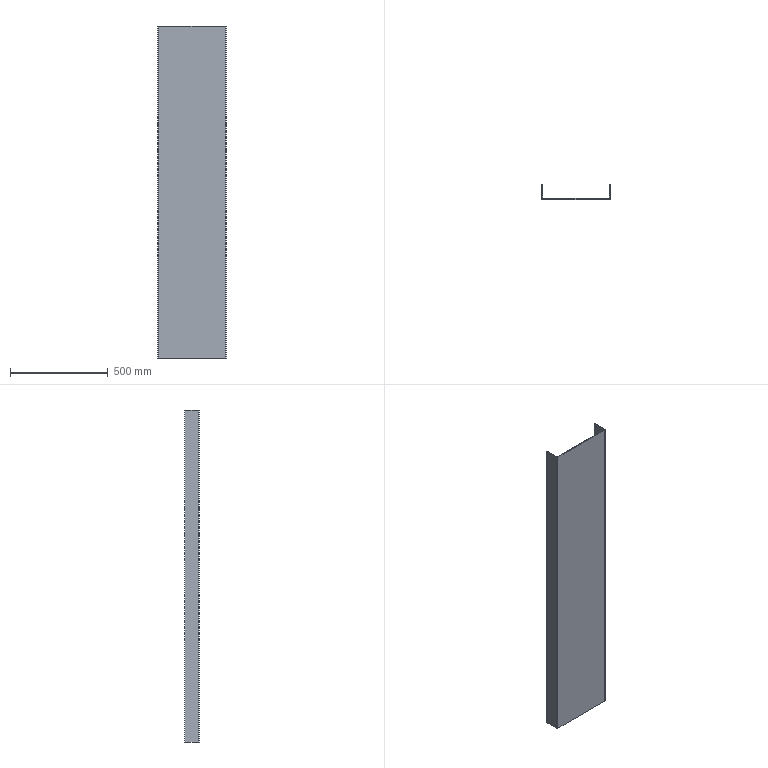Part | STEP file | Sheet metal 11 | 1 solid | 22 faces | box 350 x 75 x 1700 mm | volume 3328088 mm3 | plane 18 | cylinder 4 | commonest cylinder face diameters 2 x2 10 x2
STEP:
#1=CARTESIAN_POINT('',(-170.,-4.,850.));
#2=VERTEX_POINT('',#1);
#3=CARTESIAN_POINT('',(-170.,-4.,-850.));
#4=VERTEX_POINT('',#3);
#5=CARTESIAN_POINT('',(-170.,-4.,850.));
#6=DIRECTION('',(0.,0.,-1.));
#7=VECTOR('',#6,1000.);
#8=LINE('',#5,#7);
#9=EDGE_CURVE('',#2,#4,#8,.T.);
#10=ORIENTED_EDGE('',*,*,#9,.T.);
#11=CARTESIAN_POINT('',(170.,-4.,-850.));
#12=VERTEX_POINT('',#11);
#13=CARTESIAN_POINT('',(-175.,-4.,-850.));
#14=DIRECTION('',(-1.,0.,0.));
#15=VECTOR('',#14,1000.);
#16=LINE('',#13,#15);
#17=EDGE_CURVE('',#12,#4,#16,.T.);
#18=ORIENTED_EDGE('',*,*,#17,.F.);
#19=CARTESIAN_POINT('',(170.,-4.,850.));
#20=VERTEX_POINT('',#19);
#21=CARTESIAN_POINT('',(170.,-4.,-850.));
#22=DIRECTION('',(0.,0.,1.));
#23=VECTOR('',#22,1000.);
#24=LINE('',#21,#23);
#25=EDGE_CURVE('',#12,#20,#24,.T.);
#26=ORIENTED_EDGE('',*,*,#25,.T.);
#27=CARTESIAN_POINT('',(-175.,-4.,850.));
#28=DIRECTION('',(1.,0.,0.));
#29=VECTOR('',#28,1000.);
#30=LINE('',#27,#29);
#31=EDGE_CURVE('',#2,#20,#30,.T.);
#32=ORIENTED_EDGE('',*,*,#31,.F.);
#33=EDGE_LOOP('',(#10,#18,#26,#32));
#34=FACE_OUTER_BOUND('',#33,.T.);
#35=CARTESIAN_POINT('',(0.,-4.,0.));
#36=DIRECTION('',(0.,1.,0.));
#37=DIRECTION('',(0.,0.,1.));
#38=AXIS2_PLACEMENT_3D('',#35,#36,#37);
#39=PLANE('',#38);
#40=ADVANCED_FACE('',(#34),#39,.F.);
#41=CARTESIAN_POINT('',(170.,0.,-850.));
#42=VERTEX_POINT('',#41);
#43=CARTESIAN_POINT('',(-170.,0.,-850.));
#44=VERTEX_POINT('',#43);
#45=CARTESIAN_POINT('',(-175.,0.,-850.));
#46=DIRECTION('',(-1.,0.,0.));
#47=VECTOR('',#46,1000.);
#48=LINE('',#45,#47);
#49=EDGE_CURVE('',#42,#44,#48,.T.);
#50=ORIENTED_EDGE('',*,*,#49,.T.);
#51=CARTESIAN_POINT('',(-170.,0.,850.));
#52=VERTEX_POINT('',#51);
#53=CARTESIAN_POINT('',(-170.,0.,850.));
#54=DIRECTION('',(0.,0.,-1.));
#55=VECTOR('',#54,1000.);
#56=LINE('',#53,#55);
#57=EDGE_CURVE('',#52,#44,#56,.T.);
#58=ORIENTED_EDGE('',*,*,#57,.F.);
#59=CARTESIAN_POINT('',(170.,0.,850.));
#60=VERTEX_POINT('',#59);
#61=CARTESIAN_POINT('',(-175.,0.,850.));
#62=DIRECTION('',(1.,0.,0.));
#63=VECTOR('',#62,1000.);
#64=LINE('',#61,#63);
#65=EDGE_CURVE('',#52,#60,#64,.T.);
#66=ORIENTED_EDGE('',*,*,#65,.T.);
#67=CARTESIAN_POINT('',(170.,0.,-850.));
#68=DIRECTION('',(0.,0.,1.));
#69=VECTOR('',#68,1000.);
#70=LINE('',#67,#69);
#71=EDGE_CURVE('',#42,#60,#70,.T.);
#72=ORIENTED_EDGE('',*,*,#71,.F.);
#73=EDGE_LOOP('',(#50,#58,#66,#72));
#74=FACE_OUTER_BOUND('',#73,.T.);
#75=CARTESIAN_POINT('',(0.,0.,0.));
#76=DIRECTION('',(0.,1.,0.));
#77=DIRECTION('',(0.,0.,1.));
#78=AXIS2_PLACEMENT_3D('',#75,#76,#77);
#79=PLANE('',#78);
#80=ADVANCED_FACE('',(#74),#79,.T.);
#81=ORIENTED_EDGE('',*,*,#65,.F.);
#82=CARTESIAN_POINT('',(-170.,0.,850.));
#83=DIRECTION('',(0.,-1.,0.));
#84=VECTOR('',#83,1000.);
#85=LINE('',#82,#84);
#86=EDGE_CURVE('',#52,#2,#85,.T.);
#87=ORIENTED_EDGE('',*,*,#86,.T.);
#88=ORIENTED_EDGE('',*,*,#31,.T.);
#89=CARTESIAN_POINT('',(170.,0.,850.));
#90=DIRECTION('',(0.,-1.,0.));
#91=VECTOR('',#90,1000.);
#92=LINE('',#89,#91);
#93=EDGE_CURVE('',#60,#20,#92,.T.);
#94=ORIENTED_EDGE('',*,*,#93,.F.);
#95=EDGE_LOOP('',(#81,#87,#88,#94));
#96=FACE_OUTER_BOUND('',#95,.T.);
#97=CARTESIAN_POINT('',(-175.,-4.,850.));
#98=DIRECTION('',(0.,0.,1.));
#99=DIRECTION('',(1.,0.,0.));
#100=AXIS2_PLACEMENT_3D('',#97,#98,#99);
#101=PLANE('',#100);
#102=ADVANCED_FACE('',(#96),#101,.T.);
#103=CARTESIAN_POINT('',(-170.,0.,-850.));
#104=DIRECTION('',(0.,-1.,0.));
#105=VECTOR('',#104,1000.);
#106=LINE('',#103,#105);
#107=EDGE_CURVE('',#44,#4,#106,.T.);
#108=ORIENTED_EDGE('',*,*,#107,.F.);
#109=ORIENTED_EDGE('',*,*,#49,.F.);
#110=CARTESIAN_POINT('',(170.,0.,-850.));
#111=DIRECTION('',(0.,-1.,0.));
#112=VECTOR('',#111,1000.);
#113=LINE('',#110,#112);
#114=EDGE_CURVE('',#42,#12,#113,.T.);
#115=ORIENTED_EDGE('',*,*,#114,.T.);
#116=ORIENTED_EDGE('',*,*,#17,.T.);
#117=EDGE_LOOP('',(#108,#109,#115,#116));
#118=FACE_OUTER_BOUND('',#117,.T.);
#119=CARTESIAN_POINT('',(-175.,-4.,-850.));
#120=DIRECTION('',(0.,0.,-1.));
#121=DIRECTION('',(-1.,0.,0.));
#122=AXIS2_PLACEMENT_3D('',#119,#120,#121);
#123=PLANE('',#122);
#124=ADVANCED_FACE('',(#118),#123,.T.);
#125=CARTESIAN_POINT('',(171.,1.,850.));
#126=VERTEX_POINT('',#125);
#127=CARTESIAN_POINT('',(175.,1.,850.));
#128=VERTEX_POINT('',#127);
#129=CARTESIAN_POINT('',(175.,1.,850.));
#130=DIRECTION('',(1.,0.,0.));
#131=VECTOR('',#130,1000.);
#132=LINE('',#129,#131);
#133=EDGE_CURVE('',#126,#128,#132,.T.);
#134=ORIENTED_EDGE('',*,*,#133,.F.);
#135=CARTESIAN_POINT('',(170.,1.,850.));
#136=DIRECTION('',(0.,0.,1.));
#137=DIRECTION('',(-1.,0.,0.));
#138=AXIS2_PLACEMENT_3D('',#135,#136,#137);
#139=CIRCLE('',#138,1.);
#140=EDGE_CURVE('',#60,#126,#139,.T.);
#141=ORIENTED_EDGE('',*,*,#140,.F.);
#142=ORIENTED_EDGE('',*,*,#93,.T.);
#143=CARTESIAN_POINT('',(170.,1.,850.));
#144=DIRECTION('',(0.,0.,1.));
#145=DIRECTION('',(-1.,0.,0.));
#146=AXIS2_PLACEMENT_3D('',#143,#144,#145);
#147=CIRCLE('',#146,5.);
#148=EDGE_CURVE('',#20,#128,#147,.T.);
#149=ORIENTED_EDGE('',*,*,#148,.T.);
#150=EDGE_LOOP('',(#134,#141,#142,#149));
#151=FACE_OUTER_BOUND('',#150,.T.);
#152=CARTESIAN_POINT('',(170.,1.,850.));
#153=DIRECTION('',(0.,0.,1.));
#154=DIRECTION('',(1.,0.,0.));
#155=AXIS2_PLACEMENT_3D('',#152,#153,#154);
#156=PLANE('',#155);
#157=ADVANCED_FACE('',(#151),#156,.T.);
#158=CARTESIAN_POINT('',(171.,1.,-850.));
#159=VERTEX_POINT('',#158);
#160=CARTESIAN_POINT('',(170.,1.,-850.));
#161=DIRECTION('',(0.,0.,-1.));
#162=DIRECTION('',(-1.,0.,0.));
#163=AXIS2_PLACEMENT_3D('',#160,#161,#162);
#164=CIRCLE('',#163,1.);
#165=EDGE_CURVE('',#159,#42,#164,.T.);
#166=ORIENTED_EDGE('',*,*,#165,.F.);
#167=CARTESIAN_POINT('',(175.,1.,-850.));
#168=VERTEX_POINT('',#167);
#169=CARTESIAN_POINT('',(171.,1.,-850.));
#170=DIRECTION('',(1.,0.,0.));
#171=VECTOR('',#170,1000.);
#172=LINE('',#169,#171);
#173=EDGE_CURVE('',#159,#168,#172,.T.);
#174=ORIENTED_EDGE('',*,*,#173,.T.);
#175=CARTESIAN_POINT('',(170.,1.,-850.));
#176=DIRECTION('',(0.,0.,-1.));
#177=DIRECTION('',(-1.,0.,0.));
#178=AXIS2_PLACEMENT_3D('',#175,#176,#177);
#179=CIRCLE('',#178,5.);
#180=EDGE_CURVE('',#168,#12,#179,.T.);
#181=ORIENTED_EDGE('',*,*,#180,.T.);
#182=ORIENTED_EDGE('',*,*,#114,.F.);
#183=EDGE_LOOP('',(#166,#174,#181,#182));
#184=FACE_OUTER_BOUND('',#183,.T.);
#185=CARTESIAN_POINT('',(170.,1.,-850.));
#186=DIRECTION('',(0.,0.,1.));
#187=DIRECTION('',(1.,0.,0.));
#188=AXIS2_PLACEMENT_3D('',#185,#186,#187);
#189=PLANE('',#188);
#190=ADVANCED_FACE('',(#184),#189,.F.);
#191=ORIENTED_EDGE('',*,*,#25,.F.);
#192=ORIENTED_EDGE('',*,*,#180,.F.);
#193=CARTESIAN_POINT('',(175.,1.,0.));
#194=DIRECTION('',(0.,0.,-1.));
#195=VECTOR('',#194,1000.);
#196=LINE('',#193,#195);
#197=EDGE_CURVE('',#128,#168,#196,.T.);
#198=ORIENTED_EDGE('',*,*,#197,.F.);
#199=ORIENTED_EDGE('',*,*,#148,.F.);
#200=EDGE_LOOP('',(#191,#192,#198,#199));
#201=FACE_OUTER_BOUND('',#200,.T.);
#202=CARTESIAN_POINT('',(170.,1.,-850.));
#203=DIRECTION('',(0.,0.,-1.));
#204=DIRECTION('',(1.,0.,0.));
#205=AXIS2_PLACEMENT_3D('',#202,#203,#204);
#206=CYLINDRICAL_SURFACE('',#205,5.);
#207=ADVANCED_FACE('',(#201),#206,.T.);
#208=ORIENTED_EDGE('',*,*,#71,.T.);
#209=ORIENTED_EDGE('',*,*,#140,.T.);
#210=CARTESIAN_POINT('',(171.,1.,850.));
#211=DIRECTION('',(0.,0.,-1.));
#212=VECTOR('',#211,1000.);
#213=LINE('',#210,#212);
#214=EDGE_CURVE('',#126,#159,#213,.T.);
#215=ORIENTED_EDGE('',*,*,#214,.T.);
#216=ORIENTED_EDGE('',*,*,#165,.T.);
#217=EDGE_LOOP('',(#208,#209,#215,#216));
#218=FACE_OUTER_BOUND('',#217,.T.);
#219=CARTESIAN_POINT('',(170.,1.,-850.));
#220=DIRECTION('',(0.,0.,-1.));
#221=DIRECTION('',(1.,0.,0.));
#222=AXIS2_PLACEMENT_3D('',#219,#220,#221);
#223=CYLINDRICAL_SURFACE('',#222,1.);
#224=ADVANCED_FACE('',(#218),#223,.F.);
#225=CARTESIAN_POINT('',(175.,71.,-850.));
#226=VERTEX_POINT('',#225);
#227=CARTESIAN_POINT('',(175.,0.,-850.));
#228=DIRECTION('',(0.,-1.,0.));
#229=VECTOR('',#228,1000.);
#230=LINE('',#227,#229);
#231=EDGE_CURVE('',#226,#168,#230,.T.);
#232=ORIENTED_EDGE('',*,*,#231,.T.);
#233=ORIENTED_EDGE('',*,*,#173,.F.);
#234=CARTESIAN_POINT('',(171.,71.,-850.));
#235=VERTEX_POINT('',#234);
#236=CARTESIAN_POINT('',(171.,0.,-850.));
#237=DIRECTION('',(0.,-1.,0.));
#238=VECTOR('',#237,1000.);
#239=LINE('',#236,#238);
#240=EDGE_CURVE('',#235,#159,#239,.T.);
#241=ORIENTED_EDGE('',*,*,#240,.F.);
#242=CARTESIAN_POINT('',(175.,71.,-850.));
#243=DIRECTION('',(-1.,0.,0.));
#244=VECTOR('',#243,1000.);
#245=LINE('',#242,#244);
#246=EDGE_CURVE('',#226,#235,#245,.T.);
#247=ORIENTED_EDGE('',*,*,#246,.F.);
#248=EDGE_LOOP('',(#232,#233,#241,#247));
#249=FACE_OUTER_BOUND('',#248,.T.);
#250=CARTESIAN_POINT('',(175.,0.,-850.));
#251=DIRECTION('',(0.,0.,-1.));
#252=DIRECTION('',(-1.,0.,0.));
#253=AXIS2_PLACEMENT_3D('',#250,#251,#252);
#254=PLANE('',#253);
#255=ADVANCED_FACE('',(#249),#254,.T.);
#256=CARTESIAN_POINT('',(171.,71.,850.));
#257=VERTEX_POINT('',#256);
#258=CARTESIAN_POINT('',(171.,0.,850.));
#259=DIRECTION('',(0.,1.,0.));
#260=VECTOR('',#259,1000.);
#261=LINE('',#258,#260);
#262=EDGE_CURVE('',#126,#257,#261,.T.);
#263=ORIENTED_EDGE('',*,*,#262,.F.);
#264=ORIENTED_EDGE('',*,*,#133,.T.);
#265=CARTESIAN_POINT('',(175.,71.,850.));
#266=VERTEX_POINT('',#265);
#267=CARTESIAN_POINT('',(175.,71.,850.));
#268=DIRECTION('',(0.,1.,0.));
#269=VECTOR('',#268,1000.);
#270=LINE('',#267,#269);
#271=EDGE_CURVE('',#128,#266,#270,.T.);
#272=ORIENTED_EDGE('',*,*,#271,.T.);
#273=CARTESIAN_POINT('',(175.,71.,850.));
#274=DIRECTION('',(-1.,0.,0.));
#275=VECTOR('',#274,1000.);
#276=LINE('',#273,#275);
#277=EDGE_CURVE('',#266,#257,#276,.T.);
#278=ORIENTED_EDGE('',*,*,#277,.T.);
#279=EDGE_LOOP('',(#263,#264,#272,#278));
#280=FACE_OUTER_BOUND('',#279,.T.);
#281=CARTESIAN_POINT('',(175.,71.,850.));
#282=DIRECTION('',(0.,0.,1.));
#283=DIRECTION('',(1.,0.,0.));
#284=AXIS2_PLACEMENT_3D('',#281,#282,#283);
#285=PLANE('',#284);
#286=ADVANCED_FACE('',(#280),#285,.T.);
#287=ORIENTED_EDGE('',*,*,#271,.F.);
#288=ORIENTED_EDGE('',*,*,#197,.T.);
#289=ORIENTED_EDGE('',*,*,#231,.F.);
#290=CARTESIAN_POINT('',(175.,71.,-850.));
#291=DIRECTION('',(0.,0.,-1.));
#292=VECTOR('',#291,1000.);
#293=LINE('',#290,#292);
#294=EDGE_CURVE('',#266,#226,#293,.T.);
#295=ORIENTED_EDGE('',*,*,#294,.F.);
#296=EDGE_LOOP('',(#287,#288,#289,#295));
#297=FACE_OUTER_BOUND('',#296,.T.);
#298=CARTESIAN_POINT('',(175.,0.,0.));
#299=DIRECTION('',(1.,0.,0.));
#300=DIRECTION('',(0.,1.,0.));
#301=AXIS2_PLACEMENT_3D('',#298,#299,#300);
#302=PLANE('',#301);
#303=ADVANCED_FACE('',(#297),#302,.T.);
#304=ORIENTED_EDGE('',*,*,#214,.F.);
#305=ORIENTED_EDGE('',*,*,#262,.T.);
#306=CARTESIAN_POINT('',(171.,71.,0.));
#307=DIRECTION('',(0.,0.,-1.));
#308=VECTOR('',#307,1000.);
#309=LINE('',#306,#308);
#310=EDGE_CURVE('',#257,#235,#309,.T.);
#311=ORIENTED_EDGE('',*,*,#310,.T.);
#312=ORIENTED_EDGE('',*,*,#240,.T.);
#313=EDGE_LOOP('',(#304,#305,#311,#312));
#314=FACE_OUTER_BOUND('',#313,.T.);
#315=CARTESIAN_POINT('',(171.,0.,0.));
#316=DIRECTION('',(1.,0.,0.));
#317=DIRECTION('',(0.,1.,0.));
#318=AXIS2_PLACEMENT_3D('',#315,#316,#317);
#319=PLANE('',#318);
#320=ADVANCED_FACE('',(#314),#319,.F.);
#321=ORIENTED_EDGE('',*,*,#310,.F.);
#322=ORIENTED_EDGE('',*,*,#277,.F.);
#323=ORIENTED_EDGE('',*,*,#294,.T.);
#324=ORIENTED_EDGE('',*,*,#246,.T.);
#325=EDGE_LOOP('',(#321,#322,#323,#324));
#326=FACE_OUTER_BOUND('',#325,.T.);
#327=CARTESIAN_POINT('',(175.,71.,-850.));
#328=DIRECTION('',(0.,1.,0.));
#329=DIRECTION('',(-1.,0.,0.));
#330=AXIS2_PLACEMENT_3D('',#327,#328,#329);
#331=PLANE('',#330);
#332=ADVANCED_FACE('',(#326),#331,.T.);
#333=CARTESIAN_POINT('',(-171.,1.,-850.));
#334=VERTEX_POINT('',#333);
#335=CARTESIAN_POINT('',(-175.,1.,-850.));
#336=VERTEX_POINT('',#335);
#337=CARTESIAN_POINT('',(-175.,1.,-850.));
#338=DIRECTION('',(-1.,0.,0.));
#339=VECTOR('',#338,1000.);
#340=LINE('',#337,#339);
#341=EDGE_CURVE('',#334,#336,#340,.T.);
#342=ORIENTED_EDGE('',*,*,#341,.F.);
#343=CARTESIAN_POINT('',(-170.,1.,-850.));
#344=DIRECTION('',(0.,0.,-1.));
#345=DIRECTION('',(1.,0.,0.));
#346=AXIS2_PLACEMENT_3D('',#343,#344,#345);
#347=CIRCLE('',#346,1.);
#348=EDGE_CURVE('',#44,#334,#347,.T.);
#349=ORIENTED_EDGE('',*,*,#348,.F.);
#350=ORIENTED_EDGE('',*,*,#107,.T.);
#351=CARTESIAN_POINT('',(-170.,1.,-850.));
#352=DIRECTION('',(0.,0.,-1.));
#353=DIRECTION('',(1.,0.,0.));
#354=AXIS2_PLACEMENT_3D('',#351,#352,#353);
#355=CIRCLE('',#354,5.);
#356=EDGE_CURVE('',#4,#336,#355,.T.);
#357=ORIENTED_EDGE('',*,*,#356,.T.);
#358=EDGE_LOOP('',(#342,#349,#350,#357));
#359=FACE_OUTER_BOUND('',#358,.T.);
#360=CARTESIAN_POINT('',(-170.,1.,-850.));
#361=DIRECTION('',(0.,0.,-1.));
#362=DIRECTION('',(-1.,0.,0.));
#363=AXIS2_PLACEMENT_3D('',#360,#361,#362);
#364=PLANE('',#363);
#365=ADVANCED_FACE('',(#359),#364,.T.);
#366=CARTESIAN_POINT('',(-171.,1.,850.));
#367=VERTEX_POINT('',#366);
#368=CARTESIAN_POINT('',(-170.,1.,850.));
#369=DIRECTION('',(0.,0.,1.));
#370=DIRECTION('',(1.,0.,0.));
#371=AXIS2_PLACEMENT_3D('',#368,#369,#370);
#372=CIRCLE('',#371,1.);
#373=EDGE_CURVE('',#367,#52,#372,.T.);
#374=ORIENTED_EDGE('',*,*,#373,.F.);
#375=CARTESIAN_POINT('',(-175.,1.,850.));
#376=VERTEX_POINT('',#375);
#377=CARTESIAN_POINT('',(-171.,1.,850.));
#378=DIRECTION('',(-1.,0.,0.));
#379=VECTOR('',#378,1000.);
#380=LINE('',#377,#379);
#381=EDGE_CURVE('',#367,#376,#380,.T.);
#382=ORIENTED_EDGE('',*,*,#381,.T.);
#383=CARTESIAN_POINT('',(-170.,1.,850.));
#384=DIRECTION('',(0.,0.,1.));
#385=DIRECTION('',(1.,0.,0.));
#386=AXIS2_PLACEMENT_3D('',#383,#384,#385);
#387=CIRCLE('',#386,5.);
#388=EDGE_CURVE('',#376,#2,#387,.T.);
#389=ORIENTED_EDGE('',*,*,#388,.T.);
#390=ORIENTED_EDGE('',*,*,#86,.F.);
#391=EDGE_LOOP('',(#374,#382,#389,#390));
#392=FACE_OUTER_BOUND('',#391,.T.);
#393=CARTESIAN_POINT('',(-170.,1.,850.));
#394=DIRECTION('',(0.,0.,-1.));
#395=DIRECTION('',(-1.,0.,0.));
#396=AXIS2_PLACEMENT_3D('',#393,#394,#395);
#397=PLANE('',#396);
#398=ADVANCED_FACE('',(#392),#397,.F.);
#399=ORIENTED_EDGE('',*,*,#9,.F.);
#400=ORIENTED_EDGE('',*,*,#388,.F.);
#401=CARTESIAN_POINT('',(-175.,1.,-850.));
#402=DIRECTION('',(0.,0.,-1.));
#403=VECTOR('',#402,1000.);
#404=LINE('',#401,#403);
#405=EDGE_CURVE('',#376,#336,#404,.T.);
#406=ORIENTED_EDGE('',*,*,#405,.T.);
#407=ORIENTED_EDGE('',*,*,#356,.F.);
#408=EDGE_LOOP('',(#399,#400,#406,#407));
#409=FACE_OUTER_BOUND('',#408,.T.);
#410=CARTESIAN_POINT('',(-170.,1.,850.));
#411=DIRECTION('',(0.,0.,1.));
#412=DIRECTION('',(-1.,0.,0.));
#413=AXIS2_PLACEMENT_3D('',#410,#411,#412);
#414=CYLINDRICAL_SURFACE('',#413,5.);
#415=ADVANCED_FACE('',(#409),#414,.T.);
#416=ORIENTED_EDGE('',*,*,#57,.T.);
#417=ORIENTED_EDGE('',*,*,#348,.T.);
#418=CARTESIAN_POINT('',(-171.,1.,-850.));
#419=DIRECTION('',(0.,0.,1.));
#420=VECTOR('',#419,1000.);
#421=LINE('',#418,#420);
#422=EDGE_CURVE('',#334,#367,#421,.T.);
#423=ORIENTED_EDGE('',*,*,#422,.T.);
#424=ORIENTED_EDGE('',*,*,#373,.T.);
#425=EDGE_LOOP('',(#416,#417,#423,#424));
#426=FACE_OUTER_BOUND('',#425,.T.);
#427=CARTESIAN_POINT('',(-170.,1.,850.));
#428=DIRECTION('',(0.,0.,1.));
#429=DIRECTION('',(-1.,0.,0.));
#430=AXIS2_PLACEMENT_3D('',#427,#428,#429);
#431=CYLINDRICAL_SURFACE('',#430,1.);
#432=ADVANCED_FACE('',(#426),#431,.F.);
#433=CARTESIAN_POINT('',(-171.,71.,-850.));
#434=VERTEX_POINT('',#433);
#435=CARTESIAN_POINT('',(-171.,0.,-850.));
#436=DIRECTION('',(0.,1.,0.));
#437=VECTOR('',#436,1000.);
#438=LINE('',#435,#437);
#439=EDGE_CURVE('',#334,#434,#438,.T.);
#440=ORIENTED_EDGE('',*,*,#439,.F.);
#441=ORIENTED_EDGE('',*,*,#341,.T.);
#442=CARTESIAN_POINT('',(-175.,71.,-850.));
#443=VERTEX_POINT('',#442);
#444=CARTESIAN_POINT('',(-175.,0.,-850.));
#445=DIRECTION('',(0.,1.,0.));
#446=VECTOR('',#445,1000.);
#447=LINE('',#444,#446);
#448=EDGE_CURVE('',#336,#443,#447,.T.);
#449=ORIENTED_EDGE('',*,*,#448,.T.);
#450=CARTESIAN_POINT('',(-175.,71.,-850.));
#451=DIRECTION('',(1.,0.,0.));
#452=VECTOR('',#451,1000.);
#453=LINE('',#450,#452);
#454=EDGE_CURVE('',#443,#434,#453,.T.);
#455=ORIENTED_EDGE('',*,*,#454,.T.);
#456=EDGE_LOOP('',(#440,#441,#449,#455));
#457=FACE_OUTER_BOUND('',#456,.T.);
#458=CARTESIAN_POINT('',(-175.,0.,-850.));
#459=DIRECTION('',(0.,0.,-1.));
#460=DIRECTION('',(-1.,0.,0.));
#461=AXIS2_PLACEMENT_3D('',#458,#459,#460);
#462=PLANE('',#461);
#463=ADVANCED_FACE('',(#457),#462,.T.);
#464=CARTESIAN_POINT('',(-175.,71.,850.));
#465=VERTEX_POINT('',#464);
#466=CARTESIAN_POINT('',(-175.,71.,850.));
#467=DIRECTION('',(0.,-1.,0.));
#468=VECTOR('',#467,1000.);
#469=LINE('',#466,#468);
#470=EDGE_CURVE('',#465,#376,#469,.T.);
#471=ORIENTED_EDGE('',*,*,#470,.T.);
#472=ORIENTED_EDGE('',*,*,#381,.F.);
#473=CARTESIAN_POINT('',(-171.,71.,850.));
#474=VERTEX_POINT('',#473);
#475=CARTESIAN_POINT('',(-171.,0.,850.));
#476=DIRECTION('',(0.,-1.,0.));
#477=VECTOR('',#476,1000.);
#478=LINE('',#475,#477);
#479=EDGE_CURVE('',#474,#367,#478,.T.);
#480=ORIENTED_EDGE('',*,*,#479,.F.);
#481=CARTESIAN_POINT('',(-175.,71.,850.));
#482=DIRECTION('',(1.,0.,0.));
#483=VECTOR('',#482,1000.);
#484=LINE('',#481,#483);
#485=EDGE_CURVE('',#465,#474,#484,.T.);
#486=ORIENTED_EDGE('',*,*,#485,.F.);
#487=EDGE_LOOP('',(#471,#472,#480,#486));
#488=FACE_OUTER_BOUND('',#487,.T.);
#489=CARTESIAN_POINT('',(-175.,71.,850.));
#490=DIRECTION('',(0.,0.,1.));
#491=DIRECTION('',(1.,0.,0.));
#492=AXIS2_PLACEMENT_3D('',#489,#490,#491);
#493=PLANE('',#492);
#494=ADVANCED_FACE('',(#488),#493,.T.);
#495=ORIENTED_EDGE('',*,*,#405,.F.);
#496=ORIENTED_EDGE('',*,*,#470,.F.);
#497=CARTESIAN_POINT('',(-175.,71.,-850.));
#498=DIRECTION('',(0.,0.,1.));
#499=VECTOR('',#498,1000.);
#500=LINE('',#497,#499);
#501=EDGE_CURVE('',#443,#465,#500,.T.);
#502=ORIENTED_EDGE('',*,*,#501,.F.);
#503=ORIENTED_EDGE('',*,*,#448,.F.);
#504=EDGE_LOOP('',(#495,#496,#502,#503));
#505=FACE_OUTER_BOUND('',#504,.T.);
#506=CARTESIAN_POINT('',(-175.,0.,0.));
#507=DIRECTION('',(1.,0.,0.));
#508=DIRECTION('',(0.,1.,0.));
#509=AXIS2_PLACEMENT_3D('',#506,#507,#508);
#510=PLANE('',#509);
#511=ADVANCED_FACE('',(#505),#510,.F.);
#512=ORIENTED_EDGE('',*,*,#479,.T.);
#513=ORIENTED_EDGE('',*,*,#422,.F.);
#514=ORIENTED_EDGE('',*,*,#439,.T.);
#515=CARTESIAN_POINT('',(-171.,71.,0.));
#516=DIRECTION('',(0.,0.,1.));
#517=VECTOR('',#516,1000.);
#518=LINE('',#515,#517);
#519=EDGE_CURVE('',#434,#474,#518,.T.);
#520=ORIENTED_EDGE('',*,*,#519,.T.);
#521=EDGE_LOOP('',(#512,#513,#514,#520));
#522=FACE_OUTER_BOUND('',#521,.T.);
#523=CARTESIAN_POINT('',(-171.,0.,0.));
#524=DIRECTION('',(1.,0.,0.));
#525=DIRECTION('',(0.,1.,0.));
#526=AXIS2_PLACEMENT_3D('',#523,#524,#525);
#527=PLANE('',#526);
#528=ADVANCED_FACE('',(#522),#527,.T.);
#529=ORIENTED_EDGE('',*,*,#519,.F.);
#530=ORIENTED_EDGE('',*,*,#454,.F.);
#531=ORIENTED_EDGE('',*,*,#501,.T.);
#532=ORIENTED_EDGE('',*,*,#485,.T.);
#533=EDGE_LOOP('',(#529,#530,#531,#532));
#534=FACE_OUTER_BOUND('',#533,.T.);
#535=CARTESIAN_POINT('',(-175.,71.,-850.));
#536=DIRECTION('',(0.,1.,0.));
#537=DIRECTION('',(-1.,0.,0.));
#538=AXIS2_PLACEMENT_3D('',#535,#536,#537);
#539=PLANE('',#538);
#540=ADVANCED_FACE('',(#534),#539,.T.);
#541=CLOSED_SHELL('',(#40,#80,#102,#124,#157,#190,#207,#224,#255,#286,#303,#320,#332,#365,#398,#415,#432,#463,#494,#511,#528,#540));
#542=MANIFOLD_SOLID_BREP('',#541);
#543=CARTESIAN_POINT('',(0.,0.,0.));
#544=DIRECTION('',(0.,0.,1.));
#545=DIRECTION('',(1.,0.,0.));
#546=AXIS2_PLACEMENT_3D('',#543,#544,#545);
#547=(LENGTH_UNIT()NAMED_UNIT(*)SI_UNIT(.MILLI.,.METRE.));
#548=UNCERTAINTY_MEASURE_WITH_UNIT(LENGTH_MEASURE(0.00001),#547,'','');
#549=(NAMED_UNIT(*)PLANE_ANGLE_UNIT()SI_UNIT($,.RADIAN.));
#550=(NAMED_UNIT(*)SI_UNIT($,.STERADIAN.)SOLID_ANGLE_UNIT());
#551=(GEOMETRIC_REPRESENTATION_CONTEXT(3)GLOBAL_UNCERTAINTY_ASSIGNED_CONTEXT((#548))GLOBAL_UNIT_ASSIGNED_CONTEXT((#547,#549,#550))REPRESENTATION_CONTEXT('',''));
#552=ADVANCED_BREP_SHAPE_REPRESENTATION('',(#542,#546),#551);